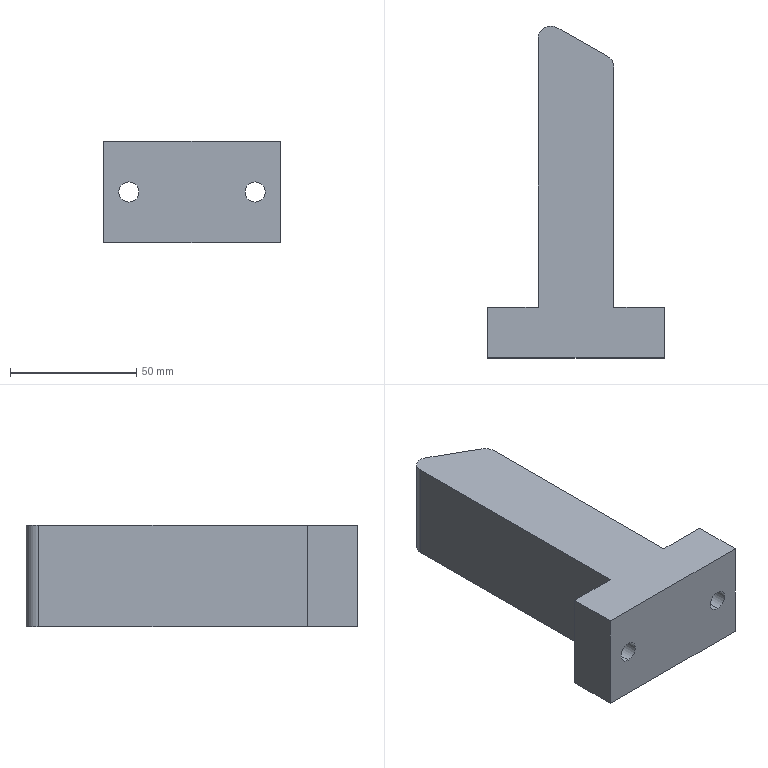Part | SolidWorks | features ICE 3, Extrusion 1, Fillet 1, MoveFace 1 | 1 solid | 22 faces | box 70 x 131.42 x 40 mm | volume 176977 mm3 | plane 12 | cylinder 10 | commonest cylinder face diameters 8 x4 18 x4 10 x2
STEP:
#1=CARTESIAN_POINT('',(-25.,10.,-9.));
#2=VERTEX_POINT('',#1);
#3=CARTESIAN_POINT('',(-25.,10.,9.));
#4=VERTEX_POINT('',#3);
#5=CARTESIAN_POINT('',(-25.,10.,0.));
#6=DIRECTION('',(0.,1.,0.));
#7=DIRECTION('',(0.,0.,1.));
#8=AXIS2_PLACEMENT_3D('',#5,#6,#7);
#9=CIRCLE('',#8,9.);
#10=EDGE_CURVE('',#2,#4,#9,.T.);
#11=ORIENTED_EDGE('',*,*,#10,.F.);
#12=CARTESIAN_POINT('',(-25.,20.,-9.));
#13=VERTEX_POINT('',#12);
#14=CARTESIAN_POINT('',(-25.,10.,-9.));
#15=DIRECTION('',(0.,1.,0.));
#16=VECTOR('',#15,1000.);
#17=LINE('',#14,#16);
#18=EDGE_CURVE('',#2,#13,#17,.T.);
#19=ORIENTED_EDGE('',*,*,#18,.T.);
#20=CARTESIAN_POINT('',(-25.,20.,9.));
#21=VERTEX_POINT('',#20);
#22=CARTESIAN_POINT('',(-25.,20.,0.));
#23=DIRECTION('',(0.,1.,0.));
#24=DIRECTION('',(0.,0.,1.));
#25=AXIS2_PLACEMENT_3D('',#22,#23,#24);
#26=CIRCLE('',#25,9.);
#27=EDGE_CURVE('',#13,#21,#26,.T.);
#28=ORIENTED_EDGE('',*,*,#27,.T.);
#29=CARTESIAN_POINT('',(-25.,10.,9.));
#30=DIRECTION('',(0.,1.,0.));
#31=VECTOR('',#30,1000.);
#32=LINE('',#29,#31);
#33=EDGE_CURVE('',#4,#21,#32,.T.);
#34=ORIENTED_EDGE('',*,*,#33,.F.);
#35=EDGE_LOOP('',(#11,#19,#28,#34));
#36=FACE_OUTER_BOUND('',#35,.T.);
#37=CARTESIAN_POINT('',(-25.,10.,0.));
#38=DIRECTION('',(0.,1.,0.));
#39=DIRECTION('',(0.,0.,1.));
#40=AXIS2_PLACEMENT_3D('',#37,#38,#39);
#41=CYLINDRICAL_SURFACE('',#40,9.);
#42=ADVANCED_FACE('',(#36),#41,.F.);
#43=CARTESIAN_POINT('',(25.,10.,-9.));
#44=VERTEX_POINT('',#43);
#45=CARTESIAN_POINT('',(25.,10.,9.));
#46=VERTEX_POINT('',#45);
#47=CARTESIAN_POINT('',(25.,10.,0.));
#48=DIRECTION('',(0.,1.,0.));
#49=DIRECTION('',(0.,0.,1.));
#50=AXIS2_PLACEMENT_3D('',#47,#48,#49);
#51=CIRCLE('',#50,9.);
#52=EDGE_CURVE('',#44,#46,#51,.T.);
#53=ORIENTED_EDGE('',*,*,#52,.F.);
#54=CARTESIAN_POINT('',(25.,20.,-9.));
#55=VERTEX_POINT('',#54);
#56=CARTESIAN_POINT('',(25.,10.,-9.));
#57=DIRECTION('',(0.,1.,0.));
#58=VECTOR('',#57,1000.);
#59=LINE('',#56,#58);
#60=EDGE_CURVE('',#44,#55,#59,.T.);
#61=ORIENTED_EDGE('',*,*,#60,.T.);
#62=CARTESIAN_POINT('',(25.,20.,9.));
#63=VERTEX_POINT('',#62);
#64=CARTESIAN_POINT('',(25.,20.,0.));
#65=DIRECTION('',(0.,1.,0.));
#66=DIRECTION('',(0.,0.,1.));
#67=AXIS2_PLACEMENT_3D('',#64,#65,#66);
#68=CIRCLE('',#67,9.);
#69=EDGE_CURVE('',#55,#63,#68,.T.);
#70=ORIENTED_EDGE('',*,*,#69,.T.);
#71=CARTESIAN_POINT('',(25.,10.,9.));
#72=DIRECTION('',(0.,1.,0.));
#73=VECTOR('',#72,1000.);
#74=LINE('',#71,#73);
#75=EDGE_CURVE('',#46,#63,#74,.T.);
#76=ORIENTED_EDGE('',*,*,#75,.F.);
#77=EDGE_LOOP('',(#53,#61,#70,#76));
#78=FACE_OUTER_BOUND('',#77,.T.);
#79=CARTESIAN_POINT('',(25.,10.,0.));
#80=DIRECTION('',(0.,1.,0.));
#81=DIRECTION('',(0.,0.,1.));
#82=AXIS2_PLACEMENT_3D('',#79,#80,#81);
#83=CYLINDRICAL_SURFACE('',#82,9.);
#84=ADVANCED_FACE('',(#78),#83,.F.);
#85=CARTESIAN_POINT('',(25.,10.,-4.));
#86=VERTEX_POINT('',#85);
#87=CARTESIAN_POINT('',(25.,10.,4.));
#88=VERTEX_POINT('',#87);
#89=CARTESIAN_POINT('',(25.,10.,0.));
#90=DIRECTION('',(0.,1.,0.));
#91=DIRECTION('',(0.,0.,1.));
#92=AXIS2_PLACEMENT_3D('',#89,#90,#91);
#93=CIRCLE('',#92,4.);
#94=EDGE_CURVE('',#86,#88,#93,.T.);
#95=ORIENTED_EDGE('',*,*,#94,.T.);
#96=CARTESIAN_POINT('',(25.,0.,4.));
#97=VERTEX_POINT('',#96);
#98=CARTESIAN_POINT('',(25.,20.,4.));
#99=DIRECTION('',(0.,-1.,0.));
#100=VECTOR('',#99,1000.);
#101=LINE('',#98,#100);
#102=EDGE_CURVE('',#88,#97,#101,.T.);
#103=ORIENTED_EDGE('',*,*,#102,.T.);
#104=CARTESIAN_POINT('',(25.,0.,-4.));
#105=VERTEX_POINT('',#104);
#106=CARTESIAN_POINT('',(25.,0.,0.));
#107=DIRECTION('',(0.,1.,0.));
#108=DIRECTION('',(0.,0.,1.));
#109=AXIS2_PLACEMENT_3D('',#106,#107,#108);
#110=CIRCLE('',#109,4.);
#111=EDGE_CURVE('',#105,#97,#110,.T.);
#112=ORIENTED_EDGE('',*,*,#111,.F.);
#113=CARTESIAN_POINT('',(25.,20.,-4.));
#114=DIRECTION('',(0.,-1.,0.));
#115=VECTOR('',#114,1000.);
#116=LINE('',#113,#115);
#117=EDGE_CURVE('',#86,#105,#116,.T.);
#118=ORIENTED_EDGE('',*,*,#117,.F.);
#119=EDGE_LOOP('',(#95,#103,#112,#118));
#120=FACE_OUTER_BOUND('',#119,.T.);
#121=CARTESIAN_POINT('',(25.,20.,0.));
#122=DIRECTION('',(0.,-1.,0.));
#123=DIRECTION('',(0.,0.,-1.));
#124=AXIS2_PLACEMENT_3D('',#121,#122,#123);
#125=CYLINDRICAL_SURFACE('',#124,4.);
#126=ADVANCED_FACE('',(#120),#125,.F.);
#127=CARTESIAN_POINT('',(-25.,10.,-4.));
#128=VERTEX_POINT('',#127);
#129=CARTESIAN_POINT('',(-25.,10.,4.));
#130=VERTEX_POINT('',#129);
#131=CARTESIAN_POINT('',(-25.,10.,0.));
#132=DIRECTION('',(0.,1.,0.));
#133=DIRECTION('',(0.,0.,1.));
#134=AXIS2_PLACEMENT_3D('',#131,#132,#133);
#135=CIRCLE('',#134,4.);
#136=EDGE_CURVE('',#128,#130,#135,.T.);
#137=ORIENTED_EDGE('',*,*,#136,.T.);
#138=CARTESIAN_POINT('',(-25.,0.,4.));
#139=VERTEX_POINT('',#138);
#140=CARTESIAN_POINT('',(-25.,20.,4.));
#141=DIRECTION('',(0.,-1.,0.));
#142=VECTOR('',#141,1000.);
#143=LINE('',#140,#142);
#144=EDGE_CURVE('',#130,#139,#143,.T.);
#145=ORIENTED_EDGE('',*,*,#144,.T.);
#146=CARTESIAN_POINT('',(-25.,0.,-4.));
#147=VERTEX_POINT('',#146);
#148=CARTESIAN_POINT('',(-25.,0.,0.));
#149=DIRECTION('',(0.,1.,0.));
#150=DIRECTION('',(0.,0.,1.));
#151=AXIS2_PLACEMENT_3D('',#148,#149,#150);
#152=CIRCLE('',#151,4.);
#153=EDGE_CURVE('',#147,#139,#152,.T.);
#154=ORIENTED_EDGE('',*,*,#153,.F.);
#155=CARTESIAN_POINT('',(-25.,20.,-4.));
#156=DIRECTION('',(0.,-1.,0.));
#157=VECTOR('',#156,1000.);
#158=LINE('',#155,#157);
#159=EDGE_CURVE('',#128,#147,#158,.T.);
#160=ORIENTED_EDGE('',*,*,#159,.F.);
#161=EDGE_LOOP('',(#137,#145,#154,#160));
#162=FACE_OUTER_BOUND('',#161,.T.);
#163=CARTESIAN_POINT('',(-25.,20.,0.));
#164=DIRECTION('',(0.,-1.,0.));
#165=DIRECTION('',(0.,0.,-1.));
#166=AXIS2_PLACEMENT_3D('',#163,#164,#165);
#167=CYLINDRICAL_SURFACE('',#166,4.);
#168=ADVANCED_FACE('',(#162),#167,.F.);
#169=ORIENTED_EDGE('',*,*,#144,.F.);
#170=CARTESIAN_POINT('',(-25.,10.,0.));
#171=DIRECTION('',(0.,1.,0.));
#172=DIRECTION('',(0.,0.,1.));
#173=AXIS2_PLACEMENT_3D('',#170,#171,#172);
#174=CIRCLE('',#173,4.);
#175=EDGE_CURVE('',#130,#128,#174,.T.);
#176=ORIENTED_EDGE('',*,*,#175,.T.);
#177=ORIENTED_EDGE('',*,*,#159,.T.);
#178=CARTESIAN_POINT('',(-25.,0.,0.));
#179=DIRECTION('',(0.,1.,0.));
#180=DIRECTION('',(0.,0.,1.));
#181=AXIS2_PLACEMENT_3D('',#178,#179,#180);
#182=CIRCLE('',#181,4.);
#183=EDGE_CURVE('',#139,#147,#182,.T.);
#184=ORIENTED_EDGE('',*,*,#183,.F.);
#185=EDGE_LOOP('',(#169,#176,#177,#184));
#186=FACE_OUTER_BOUND('',#185,.T.);
#187=CARTESIAN_POINT('',(-25.,20.,0.));
#188=DIRECTION('',(0.,-1.,0.));
#189=DIRECTION('',(0.,0.,-1.));
#190=AXIS2_PLACEMENT_3D('',#187,#188,#189);
#191=CYLINDRICAL_SURFACE('',#190,4.);
#192=ADVANCED_FACE('',(#186),#191,.F.);
#193=ORIENTED_EDGE('',*,*,#102,.F.);
#194=CARTESIAN_POINT('',(25.,10.,0.));
#195=DIRECTION('',(0.,1.,0.));
#196=DIRECTION('',(0.,0.,1.));
#197=AXIS2_PLACEMENT_3D('',#194,#195,#196);
#198=CIRCLE('',#197,4.);
#199=EDGE_CURVE('',#88,#86,#198,.T.);
#200=ORIENTED_EDGE('',*,*,#199,.T.);
#201=ORIENTED_EDGE('',*,*,#117,.T.);
#202=CARTESIAN_POINT('',(25.,0.,0.));
#203=DIRECTION('',(0.,1.,0.));
#204=DIRECTION('',(0.,0.,1.));
#205=AXIS2_PLACEMENT_3D('',#202,#203,#204);
#206=CIRCLE('',#205,4.);
#207=EDGE_CURVE('',#97,#105,#206,.T.);
#208=ORIENTED_EDGE('',*,*,#207,.F.);
#209=EDGE_LOOP('',(#193,#200,#201,#208));
#210=FACE_OUTER_BOUND('',#209,.T.);
#211=CARTESIAN_POINT('',(25.,20.,0.));
#212=DIRECTION('',(0.,-1.,0.));
#213=DIRECTION('',(0.,0.,-1.));
#214=AXIS2_PLACEMENT_3D('',#211,#212,#213);
#215=CYLINDRICAL_SURFACE('',#214,4.);
#216=ADVANCED_FACE('',(#210),#215,.F.);
#217=CARTESIAN_POINT('',(25.,20.,0.));
#218=DIRECTION('',(0.,1.,0.));
#219=DIRECTION('',(0.,0.,1.));
#220=AXIS2_PLACEMENT_3D('',#217,#218,#219);
#221=CIRCLE('',#220,9.);
#222=EDGE_CURVE('',#63,#55,#221,.T.);
#223=ORIENTED_EDGE('',*,*,#222,.F.);
#224=ORIENTED_EDGE('',*,*,#69,.F.);
#225=EDGE_LOOP('',(#223,#224));
#226=FACE_BOUND('',#225,.T.);
#227=CARTESIAN_POINT('',(15.,20.,20.));
#228=VERTEX_POINT('',#227);
#229=CARTESIAN_POINT('',(15.,20.,-20.));
#230=VERTEX_POINT('',#229);
#231=CARTESIAN_POINT('',(15.,20.,20.));
#232=DIRECTION('',(0.,0.,-1.));
#233=VECTOR('',#232,1000.);
#234=LINE('',#231,#233);
#235=EDGE_CURVE('',#228,#230,#234,.T.);
#236=ORIENTED_EDGE('',*,*,#235,.F.);
#237=CARTESIAN_POINT('',(35.,20.,20.));
#238=VERTEX_POINT('',#237);
#239=CARTESIAN_POINT('',(-35.,20.,20.));
#240=DIRECTION('',(1.,0.,0.));
#241=VECTOR('',#240,1000.);
#242=LINE('',#239,#241);
#243=EDGE_CURVE('',#228,#238,#242,.T.);
#244=ORIENTED_EDGE('',*,*,#243,.T.);
#245=CARTESIAN_POINT('',(35.,20.,-20.));
#246=VERTEX_POINT('',#245);
#247=CARTESIAN_POINT('',(35.,20.,20.));
#248=DIRECTION('',(0.,0.,-1.));
#249=VECTOR('',#248,1000.);
#250=LINE('',#247,#249);
#251=EDGE_CURVE('',#238,#246,#250,.T.);
#252=ORIENTED_EDGE('',*,*,#251,.T.);
#253=CARTESIAN_POINT('',(-35.,20.,-20.));
#254=DIRECTION('',(-1.,0.,0.));
#255=VECTOR('',#254,1000.);
#256=LINE('',#253,#255);
#257=EDGE_CURVE('',#246,#230,#256,.T.);
#258=ORIENTED_EDGE('',*,*,#257,.T.);
#259=EDGE_LOOP('',(#236,#244,#252,#258));
#260=FACE_OUTER_BOUND('',#259,.T.);
#261=CARTESIAN_POINT('',(0.,20.,0.));
#262=DIRECTION('',(0.,-1.,0.));
#263=DIRECTION('',(0.,0.,-1.));
#264=AXIS2_PLACEMENT_3D('',#261,#262,#263);
#265=PLANE('',#264);
#266=ADVANCED_FACE('',(#226,#260),#265,.F.);
#267=CARTESIAN_POINT('',(-25.,20.,0.));
#268=DIRECTION('',(0.,1.,0.));
#269=DIRECTION('',(0.,0.,1.));
#270=AXIS2_PLACEMENT_3D('',#267,#268,#269);
#271=CIRCLE('',#270,9.);
#272=EDGE_CURVE('',#21,#13,#271,.T.);
#273=ORIENTED_EDGE('',*,*,#272,.F.);
#274=ORIENTED_EDGE('',*,*,#27,.F.);
#275=EDGE_LOOP('',(#273,#274));
#276=FACE_BOUND('',#275,.T.);
#277=CARTESIAN_POINT('',(-15.,20.,-20.));
#278=VERTEX_POINT('',#277);
#279=CARTESIAN_POINT('',(-15.,20.,20.));
#280=VERTEX_POINT('',#279);
#281=CARTESIAN_POINT('',(-15.,20.,20.));
#282=DIRECTION('',(0.,0.,1.));
#283=VECTOR('',#282,1000.);
#284=LINE('',#281,#283);
#285=EDGE_CURVE('',#278,#280,#284,.T.);
#286=ORIENTED_EDGE('',*,*,#285,.F.);
#287=CARTESIAN_POINT('',(-35.,20.,-20.));
#288=VERTEX_POINT('',#287);
#289=CARTESIAN_POINT('',(-35.,20.,-20.));
#290=DIRECTION('',(-1.,0.,0.));
#291=VECTOR('',#290,1000.);
#292=LINE('',#289,#291);
#293=EDGE_CURVE('',#278,#288,#292,.T.);
#294=ORIENTED_EDGE('',*,*,#293,.T.);
#295=CARTESIAN_POINT('',(-35.,20.,20.));
#296=VERTEX_POINT('',#295);
#297=CARTESIAN_POINT('',(-35.,20.,20.));
#298=DIRECTION('',(0.,0.,1.));
#299=VECTOR('',#298,1000.);
#300=LINE('',#297,#299);
#301=EDGE_CURVE('',#288,#296,#300,.T.);
#302=ORIENTED_EDGE('',*,*,#301,.T.);
#303=CARTESIAN_POINT('',(-35.,20.,20.));
#304=DIRECTION('',(1.,0.,0.));
#305=VECTOR('',#304,1000.);
#306=LINE('',#303,#305);
#307=EDGE_CURVE('',#296,#280,#306,.T.);
#308=ORIENTED_EDGE('',*,*,#307,.T.);
#309=EDGE_LOOP('',(#286,#294,#302,#308));
#310=FACE_OUTER_BOUND('',#309,.T.);
#311=CARTESIAN_POINT('',(0.,20.,0.));
#312=DIRECTION('',(0.,-1.,0.));
#313=DIRECTION('',(0.,0.,-1.));
#314=AXIS2_PLACEMENT_3D('',#311,#312,#313);
#315=PLANE('',#314);
#316=ADVANCED_FACE('',(#276,#310),#315,.F.);
#317=ORIENTED_EDGE('',*,*,#153,.T.);
#318=ORIENTED_EDGE('',*,*,#183,.T.);
#319=EDGE_LOOP('',(#317,#318));
#320=FACE_BOUND('',#319,.T.);
#321=CARTESIAN_POINT('',(35.,0.,20.));
#322=VERTEX_POINT('',#321);
#323=CARTESIAN_POINT('',(35.,0.,-20.));
#324=VERTEX_POINT('',#323);
#325=CARTESIAN_POINT('',(35.,0.,20.));
#326=DIRECTION('',(0.,0.,-1.));
#327=VECTOR('',#326,1000.);
#328=LINE('',#325,#327);
#329=EDGE_CURVE('',#322,#324,#328,.T.);
#330=ORIENTED_EDGE('',*,*,#329,.F.);
#331=CARTESIAN_POINT('',(-35.,0.,20.));
#332=VERTEX_POINT('',#331);
#333=CARTESIAN_POINT('',(-35.,0.,20.));
#334=DIRECTION('',(1.,0.,0.));
#335=VECTOR('',#334,1000.);
#336=LINE('',#333,#335);
#337=EDGE_CURVE('',#332,#322,#336,.T.);
#338=ORIENTED_EDGE('',*,*,#337,.F.);
#339=CARTESIAN_POINT('',(-35.,0.,-20.));
#340=VERTEX_POINT('',#339);
#341=CARTESIAN_POINT('',(-35.,0.,20.));
#342=DIRECTION('',(0.,0.,1.));
#343=VECTOR('',#342,1000.);
#344=LINE('',#341,#343);
#345=EDGE_CURVE('',#340,#332,#344,.T.);
#346=ORIENTED_EDGE('',*,*,#345,.F.);
#347=CARTESIAN_POINT('',(-35.,0.,-20.));
#348=DIRECTION('',(-1.,0.,0.));
#349=VECTOR('',#348,1000.);
#350=LINE('',#347,#349);
#351=EDGE_CURVE('',#324,#340,#350,.T.);
#352=ORIENTED_EDGE('',*,*,#351,.F.);
#353=EDGE_LOOP('',(#330,#338,#346,#352));
#354=FACE_OUTER_BOUND('',#353,.T.);
#355=ORIENTED_EDGE('',*,*,#111,.T.);
#356=ORIENTED_EDGE('',*,*,#207,.T.);
#357=EDGE_LOOP('',(#355,#356));
#358=FACE_BOUND('',#357,.T.);
#359=CARTESIAN_POINT('',(0.,0.,0.));
#360=DIRECTION('',(0.,-1.,0.));
#361=DIRECTION('',(0.,0.,-1.));
#362=AXIS2_PLACEMENT_3D('',#359,#360,#361);
#363=PLANE('',#362);
#364=ADVANCED_FACE('',(#320,#354,#358),#363,.T.);
#365=ORIENTED_EDGE('',*,*,#329,.T.);
#366=CARTESIAN_POINT('',(35.,20.,-20.));
#367=DIRECTION('',(0.,-1.,0.));
#368=VECTOR('',#367,1000.);
#369=LINE('',#366,#368);
#370=EDGE_CURVE('',#246,#324,#369,.T.);
#371=ORIENTED_EDGE('',*,*,#370,.F.);
#372=ORIENTED_EDGE('',*,*,#251,.F.);
#373=CARTESIAN_POINT('',(35.,20.,20.));
#374=DIRECTION('',(0.,-1.,0.));
#375=VECTOR('',#374,1000.);
#376=LINE('',#373,#375);
#377=EDGE_CURVE('',#238,#322,#376,.T.);
#378=ORIENTED_EDGE('',*,*,#377,.T.);
#379=EDGE_LOOP('',(#365,#371,#372,#378));
#380=FACE_OUTER_BOUND('',#379,.T.);
#381=CARTESIAN_POINT('',(35.,20.,20.));
#382=DIRECTION('',(-1.,0.,0.));
#383=DIRECTION('',(0.,0.,1.));
#384=AXIS2_PLACEMENT_3D('',#381,#382,#383);
#385=PLANE('',#384);
#386=ADVANCED_FACE('',(#380),#385,.F.);
#387=CARTESIAN_POINT('',(-15.,126.42,-20.));
#388=VERTEX_POINT('',#387);
#389=CARTESIAN_POINT('',(-15.,150.,-20.));
#390=DIRECTION('',(0.,-1.,0.));
#391=VECTOR('',#390,1000.);
#392=LINE('',#389,#391);
#393=EDGE_CURVE('',#388,#278,#392,.T.);
#394=ORIENTED_EDGE('',*,*,#393,.F.);
#395=CARTESIAN_POINT('',(-7.535,130.77,-20.));
#396=VERTEX_POINT('',#395);
#397=CARTESIAN_POINT('',(-10.,126.42,-20.));
#398=DIRECTION('',(0.,0.,-1.));
#399=DIRECTION('',(1.,0.,0.));
#400=AXIS2_PLACEMENT_3D('',#397,#398,#399);
#401=CIRCLE('',#400,5.);
#402=EDGE_CURVE('',#388,#396,#401,.T.);
#403=ORIENTED_EDGE('',*,*,#402,.T.);
#404=CARTESIAN_POINT('',(12.465,119.436,-20.));
#405=VERTEX_POINT('',#404);
#406=CARTESIAN_POINT('',(25.622,111.981,-20.));
#407=DIRECTION('',(0.87,-0.493,0.));
#408=VECTOR('',#407,1000.);
#409=LINE('',#406,#408);
#410=EDGE_CURVE('',#396,#405,#409,.T.);
#411=ORIENTED_EDGE('',*,*,#410,.T.);
#412=CARTESIAN_POINT('',(15.,115.086,-20.));
#413=VERTEX_POINT('',#412);
#414=CARTESIAN_POINT('',(10.,115.086,-20.));
#415=DIRECTION('',(0.,0.,-1.));
#416=DIRECTION('',(1.,0.,0.));
#417=AXIS2_PLACEMENT_3D('',#414,#415,#416);
#418=CIRCLE('',#417,5.);
#419=EDGE_CURVE('',#405,#413,#418,.T.);
#420=ORIENTED_EDGE('',*,*,#419,.T.);
#421=CARTESIAN_POINT('',(15.,150.,-20.));
#422=DIRECTION('',(0.,-1.,0.));
#423=VECTOR('',#422,1000.);
#424=LINE('',#421,#423);
#425=EDGE_CURVE('',#413,#230,#424,.T.);
#426=ORIENTED_EDGE('',*,*,#425,.T.);
#427=ORIENTED_EDGE('',*,*,#257,.F.);
#428=ORIENTED_EDGE('',*,*,#370,.T.);
#429=ORIENTED_EDGE('',*,*,#351,.T.);
#430=CARTESIAN_POINT('',(-35.,20.,-20.));
#431=DIRECTION('',(0.,-1.,0.));
#432=VECTOR('',#431,1000.);
#433=LINE('',#430,#432);
#434=EDGE_CURVE('',#288,#340,#433,.T.);
#435=ORIENTED_EDGE('',*,*,#434,.F.);
#436=ORIENTED_EDGE('',*,*,#293,.F.);
#437=EDGE_LOOP('',(#394,#403,#411,#420,#426,#427,#428,#429,#435,#436));
#438=FACE_OUTER_BOUND('',#437,.T.);
#439=CARTESIAN_POINT('',(-35.,20.,-20.));
#440=DIRECTION('',(0.,0.,1.));
#441=DIRECTION('',(1.,0.,0.));
#442=AXIS2_PLACEMENT_3D('',#439,#440,#441);
#443=PLANE('',#442);
#444=ADVANCED_FACE('',(#438),#443,.F.);
#445=ORIENTED_EDGE('',*,*,#345,.T.);
#446=CARTESIAN_POINT('',(-35.,20.,20.));
#447=DIRECTION('',(0.,-1.,0.));
#448=VECTOR('',#447,1000.);
#449=LINE('',#446,#448);
#450=EDGE_CURVE('',#296,#332,#449,.T.);
#451=ORIENTED_EDGE('',*,*,#450,.F.);
#452=ORIENTED_EDGE('',*,*,#301,.F.);
#453=ORIENTED_EDGE('',*,*,#434,.T.);
#454=EDGE_LOOP('',(#445,#451,#452,#453));
#455=FACE_OUTER_BOUND('',#454,.T.);
#456=CARTESIAN_POINT('',(-35.,20.,20.));
#457=DIRECTION('',(1.,0.,0.));
#458=DIRECTION('',(0.,0.,-1.));
#459=AXIS2_PLACEMENT_3D('',#456,#457,#458);
#460=PLANE('',#459);
#461=ADVANCED_FACE('',(#455),#460,.F.);
#462=CARTESIAN_POINT('',(12.465,119.436,20.));
#463=VERTEX_POINT('',#462);
#464=CARTESIAN_POINT('',(-7.535,130.77,20.));
#465=VERTEX_POINT('',#464);
#466=CARTESIAN_POINT('',(25.622,111.981,20.));
#467=DIRECTION('',(-0.87,0.493,0.));
#468=VECTOR('',#467,1000.);
#469=LINE('',#466,#468);
#470=EDGE_CURVE('',#463,#465,#469,.T.);
#471=ORIENTED_EDGE('',*,*,#470,.T.);
#472=CARTESIAN_POINT('',(-15.,126.42,20.));
#473=VERTEX_POINT('',#472);
#474=CARTESIAN_POINT('',(-10.,126.42,20.));
#475=DIRECTION('',(0.,0.,1.));
#476=DIRECTION('',(-1.,0.,0.));
#477=AXIS2_PLACEMENT_3D('',#474,#475,#476);
#478=CIRCLE('',#477,5.);
#479=EDGE_CURVE('',#465,#473,#478,.T.);
#480=ORIENTED_EDGE('',*,*,#479,.T.);
#481=CARTESIAN_POINT('',(-15.,150.,20.));
#482=DIRECTION('',(0.,-1.,0.));
#483=VECTOR('',#482,1000.);
#484=LINE('',#481,#483);
#485=EDGE_CURVE('',#473,#280,#484,.T.);
#486=ORIENTED_EDGE('',*,*,#485,.T.);
#487=ORIENTED_EDGE('',*,*,#307,.F.);
#488=ORIENTED_EDGE('',*,*,#450,.T.);
#489=ORIENTED_EDGE('',*,*,#337,.T.);
#490=ORIENTED_EDGE('',*,*,#377,.F.);
#491=ORIENTED_EDGE('',*,*,#243,.F.);
#492=CARTESIAN_POINT('',(15.,115.086,20.));
#493=VERTEX_POINT('',#492);
#494=CARTESIAN_POINT('',(15.,150.,20.));
#495=DIRECTION('',(0.,-1.,0.));
#496=VECTOR('',#495,1000.);
#497=LINE('',#494,#496);
#498=EDGE_CURVE('',#493,#228,#497,.T.);
#499=ORIENTED_EDGE('',*,*,#498,.F.);
#500=CARTESIAN_POINT('',(10.,115.086,20.));
#501=DIRECTION('',(0.,0.,1.));
#502=DIRECTION('',(-1.,0.,0.));
#503=AXIS2_PLACEMENT_3D('',#500,#501,#502);
#504=CIRCLE('',#503,5.);
#505=EDGE_CURVE('',#493,#463,#504,.T.);
#506=ORIENTED_EDGE('',*,*,#505,.T.);
#507=EDGE_LOOP('',(#471,#480,#486,#487,#488,#489,#490,#491,#499,#506));
#508=FACE_OUTER_BOUND('',#507,.T.);
#509=CARTESIAN_POINT('',(-35.,20.,20.));
#510=DIRECTION('',(0.,0.,-1.));
#511=DIRECTION('',(-1.,0.,0.));
#512=AXIS2_PLACEMENT_3D('',#509,#510,#511);
#513=PLANE('',#512);
#514=ADVANCED_FACE('',(#508),#513,.F.);
#515=ORIENTED_EDGE('',*,*,#425,.F.);
#516=CARTESIAN_POINT('',(15.,115.086,20.));
#517=DIRECTION('',(0.,0.,1.));
#518=VECTOR('',#517,1000.);
#519=LINE('',#516,#518);
#520=EDGE_CURVE('',#413,#493,#519,.T.);
#521=ORIENTED_EDGE('',*,*,#520,.T.);
#522=ORIENTED_EDGE('',*,*,#498,.T.);
#523=ORIENTED_EDGE('',*,*,#235,.T.);
#524=EDGE_LOOP('',(#515,#521,#522,#523));
#525=FACE_OUTER_BOUND('',#524,.T.);
#526=CARTESIAN_POINT('',(15.,150.,20.));
#527=DIRECTION('',(-1.,0.,0.));
#528=DIRECTION('',(0.,0.,1.));
#529=AXIS2_PLACEMENT_3D('',#526,#527,#528);
#530=PLANE('',#529);
#531=ADVANCED_FACE('',(#525),#530,.F.);
#532=ORIENTED_EDGE('',*,*,#485,.F.);
#533=CARTESIAN_POINT('',(-15.,126.42,20.));
#534=DIRECTION('',(0.,0.,-1.));
#535=VECTOR('',#534,1000.);
#536=LINE('',#533,#535);
#537=EDGE_CURVE('',#473,#388,#536,.T.);
#538=ORIENTED_EDGE('',*,*,#537,.T.);
#539=ORIENTED_EDGE('',*,*,#393,.T.);
#540=ORIENTED_EDGE('',*,*,#285,.T.);
#541=EDGE_LOOP('',(#532,#538,#539,#540));
#542=FACE_OUTER_BOUND('',#541,.T.);
#543=CARTESIAN_POINT('',(-15.,150.,20.));
#544=DIRECTION('',(1.,0.,0.));
#545=DIRECTION('',(0.,0.,-1.));
#546=AXIS2_PLACEMENT_3D('',#543,#544,#545);
#547=PLANE('',#546);
#548=ADVANCED_FACE('',(#542),#547,.F.);
#549=ORIENTED_EDGE('',*,*,#410,.F.);
#550=CARTESIAN_POINT('',(-7.535,130.77,-141.));
#551=DIRECTION('',(0.,0.,1.));
#552=VECTOR('',#551,1000.);
#553=LINE('',#550,#552);
#554=EDGE_CURVE('',#396,#465,#553,.T.);
#555=ORIENTED_EDGE('',*,*,#554,.T.);
#556=ORIENTED_EDGE('',*,*,#470,.F.);
#557=CARTESIAN_POINT('',(12.465,119.436,-141.));
#558=DIRECTION('',(0.,0.,-1.));
#559=VECTOR('',#558,1000.);
#560=LINE('',#557,#559);
#561=EDGE_CURVE('',#463,#405,#560,.T.);
#562=ORIENTED_EDGE('',*,*,#561,.T.);
#563=EDGE_LOOP('',(#549,#555,#556,#562));
#564=FACE_OUTER_BOUND('',#563,.T.);
#565=CARTESIAN_POINT('',(-15.,135.,-141.));
#566=DIRECTION('',(-0.493,-0.87,0.));
#567=DIRECTION('',(0.87,-0.493,0.));
#568=AXIS2_PLACEMENT_3D('',#565,#566,#567);
#569=PLANE('',#568);
#570=ADVANCED_FACE('',(#564),#569,.F.);
#571=ORIENTED_EDGE('',*,*,#402,.F.);
#572=ORIENTED_EDGE('',*,*,#537,.F.);
#573=ORIENTED_EDGE('',*,*,#479,.F.);
#574=ORIENTED_EDGE('',*,*,#554,.F.);
#575=EDGE_LOOP('',(#571,#572,#573,#574));
#576=FACE_OUTER_BOUND('',#575,.T.);
#577=CARTESIAN_POINT('',(-10.,126.42,-141.));
#578=DIRECTION('',(0.,0.,1.));
#579=DIRECTION('',(1.,0.,0.));
#580=AXIS2_PLACEMENT_3D('',#577,#578,#579);
#581=CYLINDRICAL_SURFACE('',#580,5.);
#582=ADVANCED_FACE('',(#576),#581,.T.);
#583=ORIENTED_EDGE('',*,*,#419,.F.);
#584=ORIENTED_EDGE('',*,*,#561,.F.);
#585=ORIENTED_EDGE('',*,*,#505,.F.);
#586=ORIENTED_EDGE('',*,*,#520,.F.);
#587=EDGE_LOOP('',(#583,#584,#585,#586));
#588=FACE_OUTER_BOUND('',#587,.T.);
#589=CARTESIAN_POINT('',(10.,115.086,20.));
#590=DIRECTION('',(0.,0.,1.));
#591=DIRECTION('',(1.,0.,0.));
#592=AXIS2_PLACEMENT_3D('',#589,#590,#591);
#593=CYLINDRICAL_SURFACE('',#592,5.);
#594=ADVANCED_FACE('',(#588),#593,.T.);
#595=ORIENTED_EDGE('',*,*,#60,.F.);
#596=CARTESIAN_POINT('',(25.,10.,0.));
#597=DIRECTION('',(0.,1.,0.));
#598=DIRECTION('',(0.,0.,1.));
#599=AXIS2_PLACEMENT_3D('',#596,#597,#598);
#600=CIRCLE('',#599,9.);
#601=EDGE_CURVE('',#46,#44,#600,.T.);
#602=ORIENTED_EDGE('',*,*,#601,.F.);
#603=ORIENTED_EDGE('',*,*,#75,.T.);
#604=ORIENTED_EDGE('',*,*,#222,.T.);
#605=EDGE_LOOP('',(#595,#602,#603,#604));
#606=FACE_OUTER_BOUND('',#605,.T.);
#607=CARTESIAN_POINT('',(25.,10.,0.));
#608=DIRECTION('',(0.,1.,0.));
#609=DIRECTION('',(0.,0.,1.));
#610=AXIS2_PLACEMENT_3D('',#607,#608,#609);
#611=CYLINDRICAL_SURFACE('',#610,9.);
#612=ADVANCED_FACE('',(#606),#611,.F.);
#613=ORIENTED_EDGE('',*,*,#94,.F.);
#614=ORIENTED_EDGE('',*,*,#199,.F.);
#615=EDGE_LOOP('',(#613,#614));
#616=FACE_BOUND('',#615,.T.);
#617=ORIENTED_EDGE('',*,*,#601,.T.);
#618=ORIENTED_EDGE('',*,*,#52,.T.);
#619=EDGE_LOOP('',(#617,#618));
#620=FACE_OUTER_BOUND('',#619,.T.);
#621=CARTESIAN_POINT('',(25.,10.,0.));
#622=DIRECTION('',(0.,1.,0.));
#623=DIRECTION('',(0.,0.,1.));
#624=AXIS2_PLACEMENT_3D('',#621,#622,#623);
#625=PLANE('',#624);
#626=ADVANCED_FACE('',(#616,#620),#625,.T.);
#627=ORIENTED_EDGE('',*,*,#18,.F.);
#628=CARTESIAN_POINT('',(-25.,10.,0.));
#629=DIRECTION('',(0.,1.,0.));
#630=DIRECTION('',(0.,0.,1.));
#631=AXIS2_PLACEMENT_3D('',#628,#629,#630);
#632=CIRCLE('',#631,9.);
#633=EDGE_CURVE('',#4,#2,#632,.T.);
#634=ORIENTED_EDGE('',*,*,#633,.F.);
#635=ORIENTED_EDGE('',*,*,#33,.T.);
#636=ORIENTED_EDGE('',*,*,#272,.T.);
#637=EDGE_LOOP('',(#627,#634,#635,#636));
#638=FACE_OUTER_BOUND('',#637,.T.);
#639=CARTESIAN_POINT('',(-25.,10.,0.));
#640=DIRECTION('',(0.,1.,0.));
#641=DIRECTION('',(0.,0.,1.));
#642=AXIS2_PLACEMENT_3D('',#639,#640,#641);
#643=CYLINDRICAL_SURFACE('',#642,9.);
#644=ADVANCED_FACE('',(#638),#643,.F.);
#645=ORIENTED_EDGE('',*,*,#136,.F.);
#646=ORIENTED_EDGE('',*,*,#175,.F.);
#647=EDGE_LOOP('',(#645,#646));
#648=FACE_BOUND('',#647,.T.);
#649=ORIENTED_EDGE('',*,*,#633,.T.);
#650=ORIENTED_EDGE('',*,*,#10,.T.);
#651=EDGE_LOOP('',(#649,#650));
#652=FACE_OUTER_BOUND('',#651,.T.);
#653=CARTESIAN_POINT('',(-25.,10.,0.));
#654=DIRECTION('',(0.,1.,0.));
#655=DIRECTION('',(0.,0.,1.));
#656=AXIS2_PLACEMENT_3D('',#653,#654,#655);
#657=PLANE('',#656);
#658=ADVANCED_FACE('',(#648,#652),#657,.T.);
#659=CLOSED_SHELL('',(#42,#84,#126,#168,#192,#216,#266,#316,#364,#386,#444,#461,#514,#531,#548,#570,#582,#594,#612,#626,#644,#658));
#660=MANIFOLD_SOLID_BREP('',#659);
#661=CARTESIAN_POINT('',(0.,0.,0.));
#662=DIRECTION('',(0.,0.,1.));
#663=DIRECTION('',(1.,0.,0.));
#664=AXIS2_PLACEMENT_3D('',#661,#662,#663);
#665=(LENGTH_UNIT()NAMED_UNIT(*)SI_UNIT(.MILLI.,.METRE.));
#666=UNCERTAINTY_MEASURE_WITH_UNIT(LENGTH_MEASURE(0.00001),#665,'','');
#667=(NAMED_UNIT(*)PLANE_ANGLE_UNIT()SI_UNIT($,.RADIAN.));
#668=(NAMED_UNIT(*)SI_UNIT($,.STERADIAN.)SOLID_ANGLE_UNIT());
#669=(GEOMETRIC_REPRESENTATION_CONTEXT(3)GLOBAL_UNCERTAINTY_ASSIGNED_CONTEXT((#666))GLOBAL_UNIT_ASSIGNED_CONTEXT((#665,#667,#668))REPRESENTATION_CONTEXT('',''));
#670=ADVANCED_BREP_SHAPE_REPRESENTATION('',(#660,#664),#669);